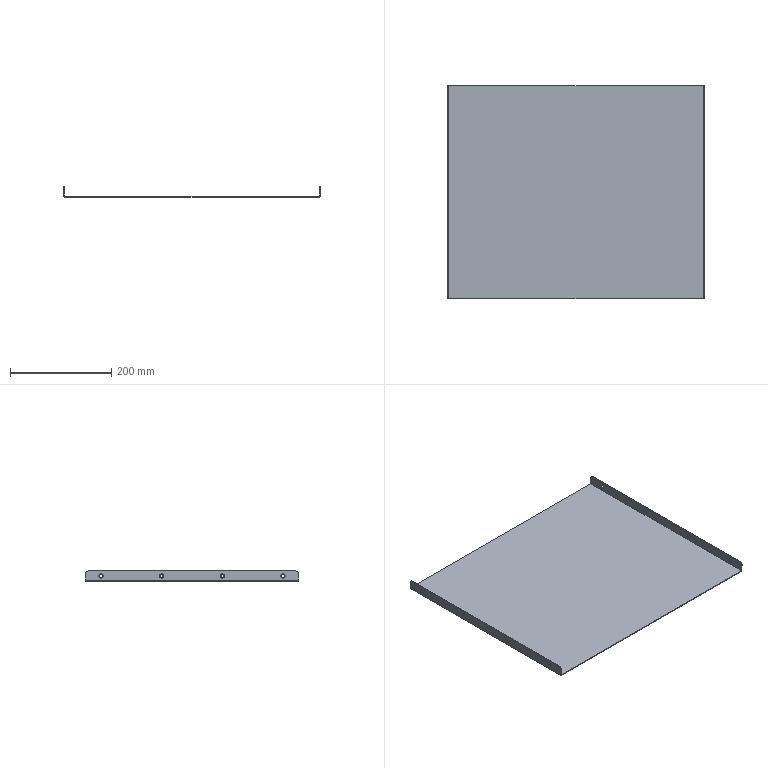Part | SolidWorks | features Chamfer 1, EdgeFlange 1, Fillet 1, FlatPattern 1, ICE 1, SMBaseFlange 1, SheetMetal 1 | 1 solid | 42 faces | box 507 x 421 x 20 mm | volume 342480 mm3 | plane 18 | cone 16 | cylinder 8 | commonest cylinder face diameters 10 x4 0.4 x2 3.4 x2
STEP:
#1=CARTESIAN_POINT('',(-253.5,180.,5.6));
#2=VERTEX_POINT('',#1);
#3=CARTESIAN_POINT('',(-253.5,180.,11.4));
#4=VERTEX_POINT('',#3);
#5=CARTESIAN_POINT('',(-253.5,180.,8.5));
#6=DIRECTION('',(-1.,0.,0.));
#7=DIRECTION('',(0.,0.,1.));
#8=AXIS2_PLACEMENT_3D('',#5,#6,#7);
#9=CIRCLE('',#8,2.9);
#10=EDGE_CURVE('',#2,#4,#9,.T.);
#11=ORIENTED_EDGE('',*,*,#10,.T.);
#12=CARTESIAN_POINT('',(-252.,180.,12.9));
#13=VERTEX_POINT('',#12);
#14=CARTESIAN_POINT('',(-253.5,180.,11.4));
#15=DIRECTION('',(0.7071,0.,0.7071));
#16=VECTOR('',#15,1000.);
#17=LINE('',#14,#16);
#18=EDGE_CURVE('',#4,#13,#17,.T.);
#19=ORIENTED_EDGE('',*,*,#18,.T.);
#20=CARTESIAN_POINT('',(-252.,180.,4.1));
#21=VERTEX_POINT('',#20);
#22=CARTESIAN_POINT('',(-252.,180.,8.5));
#23=DIRECTION('',(-1.,0.,0.));
#24=DIRECTION('',(0.,0.,-1.));
#25=AXIS2_PLACEMENT_3D('',#22,#23,#24);
#26=CIRCLE('',#25,4.4);
#27=EDGE_CURVE('',#21,#13,#26,.T.);
#28=ORIENTED_EDGE('',*,*,#27,.F.);
#29=CARTESIAN_POINT('',(-253.5,180.,5.6));
#30=DIRECTION('',(0.7071,0.,-0.7071));
#31=VECTOR('',#30,1000.);
#32=LINE('',#29,#31);
#33=EDGE_CURVE('',#2,#21,#32,.T.);
#34=ORIENTED_EDGE('',*,*,#33,.F.);
#35=EDGE_LOOP('',(#11,#19,#28,#34));
#36=FACE_OUTER_BOUND('',#35,.T.);
#37=CARTESIAN_POINT('',(-253.5,180.,8.5));
#38=DIRECTION('',(1.,0.,0.));
#39=DIRECTION('',(0.,0.,-1.));
#40=AXIS2_PLACEMENT_3D('',#37,#38,#39);
#41=CONICAL_SURFACE('',#40,2.9,0.7854);
#42=ADVANCED_FACE('',(#36),#41,.F.);
#43=CARTESIAN_POINT('',(-253.5,-180.,5.6));
#44=VERTEX_POINT('',#43);
#45=CARTESIAN_POINT('',(-253.5,-180.,11.4));
#46=VERTEX_POINT('',#45);
#47=CARTESIAN_POINT('',(-253.5,-180.,8.5));
#48=DIRECTION('',(-1.,0.,0.));
#49=DIRECTION('',(0.,0.,1.));
#50=AXIS2_PLACEMENT_3D('',#47,#48,#49);
#51=CIRCLE('',#50,2.9);
#52=EDGE_CURVE('',#44,#46,#51,.T.);
#53=ORIENTED_EDGE('',*,*,#52,.T.);
#54=CARTESIAN_POINT('',(-252.,-180.,12.9));
#55=VERTEX_POINT('',#54);
#56=CARTESIAN_POINT('',(-253.5,-180.,11.4));
#57=DIRECTION('',(0.7071,0.,0.7071));
#58=VECTOR('',#57,1000.);
#59=LINE('',#56,#58);
#60=EDGE_CURVE('',#46,#55,#59,.T.);
#61=ORIENTED_EDGE('',*,*,#60,.T.);
#62=CARTESIAN_POINT('',(-252.,-180.,4.1));
#63=VERTEX_POINT('',#62);
#64=CARTESIAN_POINT('',(-252.,-180.,8.5));
#65=DIRECTION('',(-1.,0.,0.));
#66=DIRECTION('',(0.,0.,-1.));
#67=AXIS2_PLACEMENT_3D('',#64,#65,#66);
#68=CIRCLE('',#67,4.4);
#69=EDGE_CURVE('',#63,#55,#68,.T.);
#70=ORIENTED_EDGE('',*,*,#69,.F.);
#71=CARTESIAN_POINT('',(-253.5,-180.,5.6));
#72=DIRECTION('',(0.7071,0.,-0.7071));
#73=VECTOR('',#72,1000.);
#74=LINE('',#71,#73);
#75=EDGE_CURVE('',#44,#63,#74,.T.);
#76=ORIENTED_EDGE('',*,*,#75,.F.);
#77=EDGE_LOOP('',(#53,#61,#70,#76));
#78=FACE_OUTER_BOUND('',#77,.T.);
#79=CARTESIAN_POINT('',(-253.5,-180.,8.5));
#80=DIRECTION('',(1.,0.,0.));
#81=DIRECTION('',(0.,0.,-1.));
#82=AXIS2_PLACEMENT_3D('',#79,#80,#81);
#83=CONICAL_SURFACE('',#82,2.9,0.7854);
#84=ADVANCED_FACE('',(#78),#83,.F.);
#85=CARTESIAN_POINT('',(253.5,-180.,5.6));
#86=VERTEX_POINT('',#85);
#87=CARTESIAN_POINT('',(253.5,-180.,11.4));
#88=VERTEX_POINT('',#87);
#89=CARTESIAN_POINT('',(253.5,-180.,8.5));
#90=DIRECTION('',(-1.,0.,0.));
#91=DIRECTION('',(0.,0.,1.));
#92=AXIS2_PLACEMENT_3D('',#89,#90,#91);
#93=CIRCLE('',#92,2.9);
#94=EDGE_CURVE('',#86,#88,#93,.T.);
#95=ORIENTED_EDGE('',*,*,#94,.F.);
#96=CARTESIAN_POINT('',(252.,-180.,4.1));
#97=VERTEX_POINT('',#96);
#98=CARTESIAN_POINT('',(252.,-180.,4.1));
#99=DIRECTION('',(-0.7071,0.,-0.7071));
#100=VECTOR('',#99,1000.);
#101=LINE('',#98,#100);
#102=EDGE_CURVE('',#86,#97,#101,.T.);
#103=ORIENTED_EDGE('',*,*,#102,.T.);
#104=CARTESIAN_POINT('',(252.,-180.,12.9));
#105=VERTEX_POINT('',#104);
#106=CARTESIAN_POINT('',(252.,-180.,8.5));
#107=DIRECTION('',(1.,0.,0.));
#108=DIRECTION('',(0.,0.,-1.));
#109=AXIS2_PLACEMENT_3D('',#106,#107,#108);
#110=CIRCLE('',#109,4.4);
#111=EDGE_CURVE('',#105,#97,#110,.T.);
#112=ORIENTED_EDGE('',*,*,#111,.F.);
#113=CARTESIAN_POINT('',(252.,-180.,12.9));
#114=DIRECTION('',(-0.7071,0.,0.7071));
#115=VECTOR('',#114,1000.);
#116=LINE('',#113,#115);
#117=EDGE_CURVE('',#88,#105,#116,.T.);
#118=ORIENTED_EDGE('',*,*,#117,.F.);
#119=EDGE_LOOP('',(#95,#103,#112,#118));
#120=FACE_OUTER_BOUND('',#119,.T.);
#121=CARTESIAN_POINT('',(252.,-180.,8.5));
#122=DIRECTION('',(-1.,0.,0.));
#123=DIRECTION('',(0.,0.,1.));
#124=AXIS2_PLACEMENT_3D('',#121,#122,#123);
#125=CONICAL_SURFACE('',#124,4.4,0.7854);
#126=ADVANCED_FACE('',(#120),#125,.F.);
#127=CARTESIAN_POINT('',(253.5,180.,5.6));
#128=VERTEX_POINT('',#127);
#129=CARTESIAN_POINT('',(253.5,180.,11.4));
#130=VERTEX_POINT('',#129);
#131=CARTESIAN_POINT('',(253.5,180.,8.5));
#132=DIRECTION('',(-1.,0.,0.));
#133=DIRECTION('',(0.,0.,1.));
#134=AXIS2_PLACEMENT_3D('',#131,#132,#133);
#135=CIRCLE('',#134,2.9);
#136=EDGE_CURVE('',#128,#130,#135,.T.);
#137=ORIENTED_EDGE('',*,*,#136,.F.);
#138=CARTESIAN_POINT('',(252.,180.,4.1));
#139=VERTEX_POINT('',#138);
#140=CARTESIAN_POINT('',(252.,180.,4.1));
#141=DIRECTION('',(-0.7071,0.,-0.7071));
#142=VECTOR('',#141,1000.);
#143=LINE('',#140,#142);
#144=EDGE_CURVE('',#128,#139,#143,.T.);
#145=ORIENTED_EDGE('',*,*,#144,.T.);
#146=CARTESIAN_POINT('',(252.,180.,12.9));
#147=VERTEX_POINT('',#146);
#148=CARTESIAN_POINT('',(252.,180.,8.5));
#149=DIRECTION('',(1.,0.,0.));
#150=DIRECTION('',(0.,0.,-1.));
#151=AXIS2_PLACEMENT_3D('',#148,#149,#150);
#152=CIRCLE('',#151,4.4);
#153=EDGE_CURVE('',#147,#139,#152,.T.);
#154=ORIENTED_EDGE('',*,*,#153,.F.);
#155=CARTESIAN_POINT('',(252.,180.,12.9));
#156=DIRECTION('',(-0.7071,0.,0.7071));
#157=VECTOR('',#156,1000.);
#158=LINE('',#155,#157);
#159=EDGE_CURVE('',#130,#147,#158,.T.);
#160=ORIENTED_EDGE('',*,*,#159,.F.);
#161=EDGE_LOOP('',(#137,#145,#154,#160));
#162=FACE_OUTER_BOUND('',#161,.T.);
#163=CARTESIAN_POINT('',(252.,180.,8.5));
#164=DIRECTION('',(-1.,0.,0.));
#165=DIRECTION('',(0.,0.,1.));
#166=AXIS2_PLACEMENT_3D('',#163,#164,#165);
#167=CONICAL_SURFACE('',#166,4.4,0.7854);
#168=ADVANCED_FACE('',(#162),#167,.F.);
#169=CARTESIAN_POINT('',(-253.5,60.,5.6));
#170=VERTEX_POINT('',#169);
#171=CARTESIAN_POINT('',(-253.5,60.,11.4));
#172=VERTEX_POINT('',#171);
#173=CARTESIAN_POINT('',(-253.5,60.,8.5));
#174=DIRECTION('',(-1.,0.,0.));
#175=DIRECTION('',(0.,0.,1.));
#176=AXIS2_PLACEMENT_3D('',#173,#174,#175);
#177=CIRCLE('',#176,2.9);
#178=EDGE_CURVE('',#170,#172,#177,.T.);
#179=ORIENTED_EDGE('',*,*,#178,.T.);
#180=CARTESIAN_POINT('',(-252.,60.,12.9));
#181=VERTEX_POINT('',#180);
#182=CARTESIAN_POINT('',(-253.5,60.,11.4));
#183=DIRECTION('',(0.7071,0.,0.7071));
#184=VECTOR('',#183,1000.);
#185=LINE('',#182,#184);
#186=EDGE_CURVE('',#172,#181,#185,.T.);
#187=ORIENTED_EDGE('',*,*,#186,.T.);
#188=CARTESIAN_POINT('',(-252.,60.,4.1));
#189=VERTEX_POINT('',#188);
#190=CARTESIAN_POINT('',(-252.,60.,8.5));
#191=DIRECTION('',(-1.,0.,0.));
#192=DIRECTION('',(0.,0.,-1.));
#193=AXIS2_PLACEMENT_3D('',#190,#191,#192);
#194=CIRCLE('',#193,4.4);
#195=EDGE_CURVE('',#189,#181,#194,.T.);
#196=ORIENTED_EDGE('',*,*,#195,.F.);
#197=CARTESIAN_POINT('',(-253.5,60.,5.6));
#198=DIRECTION('',(0.7071,0.,-0.7071));
#199=VECTOR('',#198,1000.);
#200=LINE('',#197,#199);
#201=EDGE_CURVE('',#170,#189,#200,.T.);
#202=ORIENTED_EDGE('',*,*,#201,.F.);
#203=EDGE_LOOP('',(#179,#187,#196,#202));
#204=FACE_OUTER_BOUND('',#203,.T.);
#205=CARTESIAN_POINT('',(-253.5,60.,8.5));
#206=DIRECTION('',(1.,0.,0.));
#207=DIRECTION('',(0.,0.,-1.));
#208=AXIS2_PLACEMENT_3D('',#205,#206,#207);
#209=CONICAL_SURFACE('',#208,2.9,0.7854);
#210=ADVANCED_FACE('',(#204),#209,.F.);
#211=CARTESIAN_POINT('',(-253.5,-60.,5.6));
#212=VERTEX_POINT('',#211);
#213=CARTESIAN_POINT('',(-253.5,-60.,11.4));
#214=VERTEX_POINT('',#213);
#215=CARTESIAN_POINT('',(-253.5,-60.,8.5));
#216=DIRECTION('',(-1.,0.,0.));
#217=DIRECTION('',(0.,0.,1.));
#218=AXIS2_PLACEMENT_3D('',#215,#216,#217);
#219=CIRCLE('',#218,2.9);
#220=EDGE_CURVE('',#212,#214,#219,.T.);
#221=ORIENTED_EDGE('',*,*,#220,.T.);
#222=CARTESIAN_POINT('',(-252.,-60.,12.9));
#223=VERTEX_POINT('',#222);
#224=CARTESIAN_POINT('',(-253.5,-60.,11.4));
#225=DIRECTION('',(0.7071,0.,0.7071));
#226=VECTOR('',#225,1000.);
#227=LINE('',#224,#226);
#228=EDGE_CURVE('',#214,#223,#227,.T.);
#229=ORIENTED_EDGE('',*,*,#228,.T.);
#230=CARTESIAN_POINT('',(-252.,-60.,4.1));
#231=VERTEX_POINT('',#230);
#232=CARTESIAN_POINT('',(-252.,-60.,8.5));
#233=DIRECTION('',(-1.,0.,0.));
#234=DIRECTION('',(0.,0.,-1.));
#235=AXIS2_PLACEMENT_3D('',#232,#233,#234);
#236=CIRCLE('',#235,4.4);
#237=EDGE_CURVE('',#231,#223,#236,.T.);
#238=ORIENTED_EDGE('',*,*,#237,.F.);
#239=CARTESIAN_POINT('',(-253.5,-60.,5.6));
#240=DIRECTION('',(0.7071,0.,-0.7071));
#241=VECTOR('',#240,1000.);
#242=LINE('',#239,#241);
#243=EDGE_CURVE('',#212,#231,#242,.T.);
#244=ORIENTED_EDGE('',*,*,#243,.F.);
#245=EDGE_LOOP('',(#221,#229,#238,#244));
#246=FACE_OUTER_BOUND('',#245,.T.);
#247=CARTESIAN_POINT('',(-253.5,-60.,8.5));
#248=DIRECTION('',(1.,0.,0.));
#249=DIRECTION('',(0.,0.,-1.));
#250=AXIS2_PLACEMENT_3D('',#247,#248,#249);
#251=CONICAL_SURFACE('',#250,2.9,0.7854);
#252=ADVANCED_FACE('',(#246),#251,.F.);
#253=CARTESIAN_POINT('',(253.5,60.,5.6));
#254=VERTEX_POINT('',#253);
#255=CARTESIAN_POINT('',(253.5,60.,11.4));
#256=VERTEX_POINT('',#255);
#257=CARTESIAN_POINT('',(253.5,60.,8.5));
#258=DIRECTION('',(-1.,0.,0.));
#259=DIRECTION('',(0.,0.,1.));
#260=AXIS2_PLACEMENT_3D('',#257,#258,#259);
#261=CIRCLE('',#260,2.9);
#262=EDGE_CURVE('',#254,#256,#261,.T.);
#263=ORIENTED_EDGE('',*,*,#262,.F.);
#264=CARTESIAN_POINT('',(252.,60.,4.1));
#265=VERTEX_POINT('',#264);
#266=CARTESIAN_POINT('',(252.,60.,4.1));
#267=DIRECTION('',(-0.7071,0.,-0.7071));
#268=VECTOR('',#267,1000.);
#269=LINE('',#266,#268);
#270=EDGE_CURVE('',#254,#265,#269,.T.);
#271=ORIENTED_EDGE('',*,*,#270,.T.);
#272=CARTESIAN_POINT('',(252.,60.,12.9));
#273=VERTEX_POINT('',#272);
#274=CARTESIAN_POINT('',(252.,60.,8.5));
#275=DIRECTION('',(1.,0.,0.));
#276=DIRECTION('',(0.,0.,-1.));
#277=AXIS2_PLACEMENT_3D('',#274,#275,#276);
#278=CIRCLE('',#277,4.4);
#279=EDGE_CURVE('',#273,#265,#278,.T.);
#280=ORIENTED_EDGE('',*,*,#279,.F.);
#281=CARTESIAN_POINT('',(252.,60.,12.9));
#282=DIRECTION('',(-0.7071,0.,0.7071));
#283=VECTOR('',#282,1000.);
#284=LINE('',#281,#283);
#285=EDGE_CURVE('',#256,#273,#284,.T.);
#286=ORIENTED_EDGE('',*,*,#285,.F.);
#287=EDGE_LOOP('',(#263,#271,#280,#286));
#288=FACE_OUTER_BOUND('',#287,.T.);
#289=CARTESIAN_POINT('',(252.,60.,8.5));
#290=DIRECTION('',(-1.,0.,0.));
#291=DIRECTION('',(0.,0.,1.));
#292=AXIS2_PLACEMENT_3D('',#289,#290,#291);
#293=CONICAL_SURFACE('',#292,4.4,0.7854);
#294=ADVANCED_FACE('',(#288),#293,.F.);
#295=CARTESIAN_POINT('',(252.,-60.,11.4));
#296=VERTEX_POINT('',#295);
#297=CARTESIAN_POINT('',(252.,-60.,5.6));
#298=VERTEX_POINT('',#297);
#299=CARTESIAN_POINT('',(252.,-60.,8.5));
#300=DIRECTION('',(1.,0.,0.));
#301=DIRECTION('',(0.,0.,-1.));
#302=AXIS2_PLACEMENT_3D('',#299,#300,#301);
#303=CIRCLE('',#302,2.9);
#304=EDGE_CURVE('',#296,#298,#303,.T.);
#305=ORIENTED_EDGE('',*,*,#304,.F.);
#306=CARTESIAN_POINT('',(253.5,-60.,12.9));
#307=VERTEX_POINT('',#306);
#308=CARTESIAN_POINT('',(253.5,-60.,12.9));
#309=DIRECTION('',(0.7071,0.,0.7071));
#310=VECTOR('',#309,1000.);
#311=LINE('',#308,#310);
#312=EDGE_CURVE('',#296,#307,#311,.T.);
#313=ORIENTED_EDGE('',*,*,#312,.T.);
#314=CARTESIAN_POINT('',(253.5,-60.,4.1));
#315=VERTEX_POINT('',#314);
#316=CARTESIAN_POINT('',(253.5,-60.,8.5));
#317=DIRECTION('',(-1.,0.,0.));
#318=DIRECTION('',(0.,0.,-1.));
#319=AXIS2_PLACEMENT_3D('',#316,#317,#318);
#320=CIRCLE('',#319,4.4);
#321=EDGE_CURVE('',#315,#307,#320,.T.);
#322=ORIENTED_EDGE('',*,*,#321,.F.);
#323=CARTESIAN_POINT('',(253.5,-60.,4.1));
#324=DIRECTION('',(0.7071,0.,-0.7071));
#325=VECTOR('',#324,1000.);
#326=LINE('',#323,#325);
#327=EDGE_CURVE('',#298,#315,#326,.T.);
#328=ORIENTED_EDGE('',*,*,#327,.F.);
#329=EDGE_LOOP('',(#305,#313,#322,#328));
#330=FACE_OUTER_BOUND('',#329,.T.);
#331=CARTESIAN_POINT('',(253.5,-60.,8.5));
#332=DIRECTION('',(1.,0.,0.));
#333=DIRECTION('',(0.,0.,-1.));
#334=AXIS2_PLACEMENT_3D('',#331,#332,#333);
#335=CONICAL_SURFACE('',#334,4.4,0.7854);
#336=ADVANCED_FACE('',(#330),#335,.F.);
#337=CARTESIAN_POINT('',(-251.8,-210.5,-1.5));
#338=VERTEX_POINT('',#337);
#339=CARTESIAN_POINT('',(-251.8,210.5,-1.5));
#340=VERTEX_POINT('',#339);
#341=CARTESIAN_POINT('',(-251.8,-210.5,-1.5));
#342=DIRECTION('',(0.,1.,0.));
#343=VECTOR('',#342,1000.);
#344=LINE('',#341,#343);
#345=EDGE_CURVE('',#338,#340,#344,.T.);
#346=ORIENTED_EDGE('',*,*,#345,.T.);
#347=CARTESIAN_POINT('',(251.8,210.5,-1.5));
#348=VERTEX_POINT('',#347);
#349=CARTESIAN_POINT('',(-253.5,210.5,-1.5));
#350=DIRECTION('',(-1.,0.,0.));
#351=VECTOR('',#350,1000.);
#352=LINE('',#349,#351);
#353=EDGE_CURVE('',#348,#340,#352,.T.);
#354=ORIENTED_EDGE('',*,*,#353,.F.);
#355=CARTESIAN_POINT('',(251.8,-210.5,-1.5));
#356=VERTEX_POINT('',#355);
#357=CARTESIAN_POINT('',(251.8,210.5,-1.5));
#358=DIRECTION('',(0.,-1.,0.));
#359=VECTOR('',#358,1000.);
#360=LINE('',#357,#359);
#361=EDGE_CURVE('',#348,#356,#360,.T.);
#362=ORIENTED_EDGE('',*,*,#361,.T.);
#363=CARTESIAN_POINT('',(-253.5,-210.5,-1.5));
#364=DIRECTION('',(1.,0.,0.));
#365=VECTOR('',#364,1000.);
#366=LINE('',#363,#365);
#367=EDGE_CURVE('',#338,#356,#366,.T.);
#368=ORIENTED_EDGE('',*,*,#367,.F.);
#369=EDGE_LOOP('',(#346,#354,#362,#368));
#370=FACE_OUTER_BOUND('',#369,.T.);
#371=CARTESIAN_POINT('',(0.,0.,-1.5));
#372=DIRECTION('',(0.,0.,1.));
#373=DIRECTION('',(1.,0.,0.));
#374=AXIS2_PLACEMENT_3D('',#371,#372,#373);
#375=PLANE('',#374);
#376=ADVANCED_FACE('',(#370),#375,.F.);
#377=CARTESIAN_POINT('',(251.8,210.5,0.));
#378=VERTEX_POINT('',#377);
#379=CARTESIAN_POINT('',(-251.8,210.5,0.));
#380=VERTEX_POINT('',#379);
#381=CARTESIAN_POINT('',(-253.5,210.5,0.));
#382=DIRECTION('',(-1.,0.,0.));
#383=VECTOR('',#382,1000.);
#384=LINE('',#381,#383);
#385=EDGE_CURVE('',#378,#380,#384,.T.);
#386=ORIENTED_EDGE('',*,*,#385,.T.);
#387=CARTESIAN_POINT('',(-251.8,-210.5,0.));
#388=VERTEX_POINT('',#387);
#389=CARTESIAN_POINT('',(-251.8,-210.5,0.));
#390=DIRECTION('',(0.,1.,0.));
#391=VECTOR('',#390,1000.);
#392=LINE('',#389,#391);
#393=EDGE_CURVE('',#388,#380,#392,.T.);
#394=ORIENTED_EDGE('',*,*,#393,.F.);
#395=CARTESIAN_POINT('',(251.8,-210.5,0.));
#396=VERTEX_POINT('',#395);
#397=CARTESIAN_POINT('',(-253.5,-210.5,0.));
#398=DIRECTION('',(1.,0.,0.));
#399=VECTOR('',#398,1000.);
#400=LINE('',#397,#399);
#401=EDGE_CURVE('',#388,#396,#400,.T.);
#402=ORIENTED_EDGE('',*,*,#401,.T.);
#403=CARTESIAN_POINT('',(251.8,210.5,0.));
#404=DIRECTION('',(0.,-1.,0.));
#405=VECTOR('',#404,1000.);
#406=LINE('',#403,#405);
#407=EDGE_CURVE('',#378,#396,#406,.T.);
#408=ORIENTED_EDGE('',*,*,#407,.F.);
#409=EDGE_LOOP('',(#386,#394,#402,#408));
#410=FACE_OUTER_BOUND('',#409,.T.);
#411=CARTESIAN_POINT('',(0.,0.,0.));
#412=DIRECTION('',(0.,0.,1.));
#413=DIRECTION('',(1.,0.,0.));
#414=AXIS2_PLACEMENT_3D('',#411,#412,#413);
#415=PLANE('',#414);
#416=ADVANCED_FACE('',(#410),#415,.T.);
#417=ORIENTED_EDGE('',*,*,#401,.F.);
#418=CARTESIAN_POINT('',(-251.8,-210.5,0.));
#419=DIRECTION('',(0.,0.,-1.));
#420=VECTOR('',#419,1000.);
#421=LINE('',#418,#420);
#422=EDGE_CURVE('',#388,#338,#421,.T.);
#423=ORIENTED_EDGE('',*,*,#422,.T.);
#424=ORIENTED_EDGE('',*,*,#367,.T.);
#425=CARTESIAN_POINT('',(251.8,-210.5,0.));
#426=DIRECTION('',(0.,0.,-1.));
#427=VECTOR('',#426,1000.);
#428=LINE('',#425,#427);
#429=EDGE_CURVE('',#396,#356,#428,.T.);
#430=ORIENTED_EDGE('',*,*,#429,.F.);
#431=EDGE_LOOP('',(#417,#423,#424,#430));
#432=FACE_OUTER_BOUND('',#431,.T.);
#433=CARTESIAN_POINT('',(-253.5,-210.5,-1.5));
#434=DIRECTION('',(0.,-1.,0.));
#435=DIRECTION('',(0.,0.,-1.));
#436=AXIS2_PLACEMENT_3D('',#433,#434,#435);
#437=PLANE('',#436);
#438=ADVANCED_FACE('',(#432),#437,.T.);
#439=CARTESIAN_POINT('',(-251.8,210.5,0.));
#440=DIRECTION('',(0.,0.,-1.));
#441=VECTOR('',#440,1000.);
#442=LINE('',#439,#441);
#443=EDGE_CURVE('',#380,#340,#442,.T.);
#444=ORIENTED_EDGE('',*,*,#443,.F.);
#445=ORIENTED_EDGE('',*,*,#385,.F.);
#446=CARTESIAN_POINT('',(251.8,210.5,0.));
#447=DIRECTION('',(0.,0.,-1.));
#448=VECTOR('',#447,1000.);
#449=LINE('',#446,#448);
#450=EDGE_CURVE('',#378,#348,#449,.T.);
#451=ORIENTED_EDGE('',*,*,#450,.T.);
#452=ORIENTED_EDGE('',*,*,#353,.T.);
#453=EDGE_LOOP('',(#444,#445,#451,#452));
#454=FACE_OUTER_BOUND('',#453,.T.);
#455=CARTESIAN_POINT('',(-253.5,210.5,-1.5));
#456=DIRECTION('',(0.,1.,0.));
#457=DIRECTION('',(0.,0.,1.));
#458=AXIS2_PLACEMENT_3D('',#455,#456,#457);
#459=PLANE('',#458);
#460=ADVANCED_FACE('',(#454),#459,.T.);
#461=CARTESIAN_POINT('',(252.,-210.5,0.2));
#462=VERTEX_POINT('',#461);
#463=CARTESIAN_POINT('',(253.5,-210.5,0.2));
#464=VERTEX_POINT('',#463);
#465=CARTESIAN_POINT('',(253.5,-210.5,0.2));
#466=DIRECTION('',(1.,0.,0.));
#467=VECTOR('',#466,1000.);
#468=LINE('',#465,#467);
#469=EDGE_CURVE('',#462,#464,#468,.T.);
#470=ORIENTED_EDGE('',*,*,#469,.F.);
#471=CARTESIAN_POINT('',(251.8,-210.5,0.2));
#472=DIRECTION('',(0.,-1.,0.));
#473=DIRECTION('',(0.,0.,1.));
#474=AXIS2_PLACEMENT_3D('',#471,#472,#473);
#475=CIRCLE('',#474,0.2);
#476=EDGE_CURVE('',#396,#462,#475,.T.);
#477=ORIENTED_EDGE('',*,*,#476,.F.);
#478=ORIENTED_EDGE('',*,*,#429,.T.);
#479=CARTESIAN_POINT('',(251.8,-210.5,0.2));
#480=DIRECTION('',(0.,-1.,0.));
#481=DIRECTION('',(0.,0.,1.));
#482=AXIS2_PLACEMENT_3D('',#479,#480,#481);
#483=CIRCLE('',#482,1.7);
#484=EDGE_CURVE('',#356,#464,#483,.T.);
#485=ORIENTED_EDGE('',*,*,#484,.T.);
#486=EDGE_LOOP('',(#470,#477,#478,#485));
#487=FACE_OUTER_BOUND('',#486,.T.);
#488=CARTESIAN_POINT('',(251.8,-210.5,0.2));
#489=DIRECTION('',(0.,-1.,0.));
#490=DIRECTION('',(0.,0.,-1.));
#491=AXIS2_PLACEMENT_3D('',#488,#489,#490);
#492=PLANE('',#491);
#493=ADVANCED_FACE('',(#487),#492,.T.);
#494=CARTESIAN_POINT('',(252.,210.5,0.2));
#495=VERTEX_POINT('',#494);
#496=CARTESIAN_POINT('',(251.8,210.5,0.2));
#497=DIRECTION('',(0.,1.,0.));
#498=DIRECTION('',(0.,0.,1.));
#499=AXIS2_PLACEMENT_3D('',#496,#497,#498);
#500=CIRCLE('',#499,0.2);
#501=EDGE_CURVE('',#495,#378,#500,.T.);
#502=ORIENTED_EDGE('',*,*,#501,.F.);
#503=CARTESIAN_POINT('',(253.5,210.5,0.2));
#504=VERTEX_POINT('',#503);
#505=CARTESIAN_POINT('',(252.,210.5,0.2));
#506=DIRECTION('',(1.,0.,0.));
#507=VECTOR('',#506,1000.);
#508=LINE('',#505,#507);
#509=EDGE_CURVE('',#495,#504,#508,.T.);
#510=ORIENTED_EDGE('',*,*,#509,.T.);
#511=CARTESIAN_POINT('',(251.8,210.5,0.2));
#512=DIRECTION('',(0.,1.,0.));
#513=DIRECTION('',(0.,0.,1.));
#514=AXIS2_PLACEMENT_3D('',#511,#512,#513);
#515=CIRCLE('',#514,1.7);
#516=EDGE_CURVE('',#504,#348,#515,.T.);
#517=ORIENTED_EDGE('',*,*,#516,.T.);
#518=ORIENTED_EDGE('',*,*,#450,.F.);
#519=EDGE_LOOP('',(#502,#510,#517,#518));
#520=FACE_OUTER_BOUND('',#519,.T.);
#521=CARTESIAN_POINT('',(251.8,210.5,0.2));
#522=DIRECTION('',(0.,-1.,0.));
#523=DIRECTION('',(0.,0.,-1.));
#524=AXIS2_PLACEMENT_3D('',#521,#522,#523);
#525=PLANE('',#524);
#526=ADVANCED_FACE('',(#520),#525,.F.);
#527=ORIENTED_EDGE('',*,*,#361,.F.);
#528=ORIENTED_EDGE('',*,*,#516,.F.);
#529=CARTESIAN_POINT('',(253.5,0.,0.2));
#530=DIRECTION('',(0.,1.,0.));
#531=VECTOR('',#530,1000.);
#532=LINE('',#529,#531);
#533=EDGE_CURVE('',#464,#504,#532,.T.);
#534=ORIENTED_EDGE('',*,*,#533,.F.);
#535=ORIENTED_EDGE('',*,*,#484,.F.);
#536=EDGE_LOOP('',(#527,#528,#534,#535));
#537=FACE_OUTER_BOUND('',#536,.T.);
#538=CARTESIAN_POINT('',(251.8,210.5,0.2));
#539=DIRECTION('',(0.,1.,0.));
#540=DIRECTION('',(1.,0.,0.));
#541=AXIS2_PLACEMENT_3D('',#538,#539,#540);
#542=CYLINDRICAL_SURFACE('',#541,1.7);
#543=ADVANCED_FACE('',(#537),#542,.T.);
#544=ORIENTED_EDGE('',*,*,#407,.T.);
#545=ORIENTED_EDGE('',*,*,#476,.T.);
#546=CARTESIAN_POINT('',(252.,-210.5,0.2));
#547=DIRECTION('',(0.,1.,0.));
#548=VECTOR('',#547,1000.);
#549=LINE('',#546,#548);
#550=EDGE_CURVE('',#462,#495,#549,.T.);
#551=ORIENTED_EDGE('',*,*,#550,.T.);
#552=ORIENTED_EDGE('',*,*,#501,.T.);
#553=EDGE_LOOP('',(#544,#545,#551,#552));
#554=FACE_OUTER_BOUND('',#553,.T.);
#555=CARTESIAN_POINT('',(251.8,210.5,0.2));
#556=DIRECTION('',(0.,1.,0.));
#557=DIRECTION('',(1.,0.,0.));
#558=AXIS2_PLACEMENT_3D('',#555,#556,#557);
#559=CYLINDRICAL_SURFACE('',#558,0.2);
#560=ADVANCED_FACE('',(#554),#559,.F.);
#561=CARTESIAN_POINT('',(252.,210.5,13.5));
#562=VERTEX_POINT('',#561);
#563=CARTESIAN_POINT('',(252.,210.5,0.));
#564=DIRECTION('',(0.,0.,-1.));
#565=VECTOR('',#564,1000.);
#566=LINE('',#563,#565);
#567=EDGE_CURVE('',#562,#495,#566,.T.);
#568=ORIENTED_EDGE('',*,*,#567,.F.);
#569=CARTESIAN_POINT('',(253.5,210.5,13.5));
#570=VERTEX_POINT('',#569);
#571=CARTESIAN_POINT('',(253.5,210.5,13.5));
#572=DIRECTION('',(1.,0.,0.));
#573=VECTOR('',#572,1000.);
#574=LINE('',#571,#573);
#575=EDGE_CURVE('',#562,#570,#574,.T.);
#576=ORIENTED_EDGE('',*,*,#575,.T.);
#577=CARTESIAN_POINT('',(253.5,210.5,0.));
#578=DIRECTION('',(0.,0.,-1.));
#579=VECTOR('',#578,1000.);
#580=LINE('',#577,#579);
#581=EDGE_CURVE('',#570,#504,#580,.T.);
#582=ORIENTED_EDGE('',*,*,#581,.T.);
#583=ORIENTED_EDGE('',*,*,#509,.F.);
#584=EDGE_LOOP('',(#568,#576,#582,#583));
#585=FACE_OUTER_BOUND('',#584,.T.);
#586=CARTESIAN_POINT('',(253.5,210.5,0.));
#587=DIRECTION('',(0.,1.,0.));
#588=DIRECTION('',(0.,0.,1.));
#589=AXIS2_PLACEMENT_3D('',#586,#587,#588);
#590=PLANE('',#589);
#591=ADVANCED_FACE('',(#585),#590,.T.);
#592=CARTESIAN_POINT('',(253.5,-210.5,13.5));
#593=VERTEX_POINT('',#592);
#594=CARTESIAN_POINT('',(253.5,-210.5,18.5));
#595=DIRECTION('',(0.,0.,1.));
#596=VECTOR('',#595,1000.);
#597=LINE('',#594,#596);
#598=EDGE_CURVE('',#464,#593,#597,.T.);
#599=ORIENTED_EDGE('',*,*,#598,.T.);
#600=CARTESIAN_POINT('',(252.,-210.5,13.5));
#601=VERTEX_POINT('',#600);
#602=CARTESIAN_POINT('',(253.5,-210.5,13.5));
#603=DIRECTION('',(-1.,0.,0.));
#604=VECTOR('',#603,1000.);
#605=LINE('',#602,#604);
#606=EDGE_CURVE('',#593,#601,#605,.T.);
#607=ORIENTED_EDGE('',*,*,#606,.T.);
#608=CARTESIAN_POINT('',(252.,-210.5,0.));
#609=DIRECTION('',(0.,0.,1.));
#610=VECTOR('',#609,1000.);
#611=LINE('',#608,#610);
#612=EDGE_CURVE('',#462,#601,#611,.T.);
#613=ORIENTED_EDGE('',*,*,#612,.F.);
#614=ORIENTED_EDGE('',*,*,#469,.T.);
#615=EDGE_LOOP('',(#599,#607,#613,#614));
#616=FACE_OUTER_BOUND('',#615,.T.);
#617=CARTESIAN_POINT('',(253.5,-210.5,18.5));
#618=DIRECTION('',(0.,-1.,0.));
#619=DIRECTION('',(0.,0.,-1.));
#620=AXIS2_PLACEMENT_3D('',#617,#618,#619);
#621=PLANE('',#620);
#622=ADVANCED_FACE('',(#616),#621,.T.);
#623=ORIENTED_EDGE('',*,*,#321,.T.);
#624=CARTESIAN_POINT('',(253.5,-60.,8.5));
#625=DIRECTION('',(-1.,0.,0.));
#626=DIRECTION('',(0.,0.,-1.));
#627=AXIS2_PLACEMENT_3D('',#624,#625,#626);
#628=CIRCLE('',#627,4.4);
#629=EDGE_CURVE('',#307,#315,#628,.T.);
#630=ORIENTED_EDGE('',*,*,#629,.T.);
#631=EDGE_LOOP('',(#623,#630));
#632=FACE_BOUND('',#631,.T.);
#633=CARTESIAN_POINT('',(253.5,-180.,8.5));
#634=DIRECTION('',(-1.,0.,0.));
#635=DIRECTION('',(0.,0.,1.));
#636=AXIS2_PLACEMENT_3D('',#633,#634,#635);
#637=CIRCLE('',#636,2.9);
#638=EDGE_CURVE('',#88,#86,#637,.T.);
#639=ORIENTED_EDGE('',*,*,#638,.T.);
#640=ORIENTED_EDGE('',*,*,#94,.T.);
#641=EDGE_LOOP('',(#639,#640));
#642=FACE_BOUND('',#641,.T.);
#643=CARTESIAN_POINT('',(253.5,60.,8.5));
#644=DIRECTION('',(-1.,0.,0.));
#645=DIRECTION('',(0.,0.,1.));
#646=AXIS2_PLACEMENT_3D('',#643,#644,#645);
#647=CIRCLE('',#646,2.9);
#648=EDGE_CURVE('',#256,#254,#647,.T.);
#649=ORIENTED_EDGE('',*,*,#648,.T.);
#650=ORIENTED_EDGE('',*,*,#262,.T.);
#651=EDGE_LOOP('',(#649,#650));
#652=FACE_BOUND('',#651,.T.);
#653=CARTESIAN_POINT('',(253.5,180.,8.5));
#654=DIRECTION('',(-1.,0.,0.));
#655=DIRECTION('',(0.,0.,1.));
#656=AXIS2_PLACEMENT_3D('',#653,#654,#655);
#657=CIRCLE('',#656,2.9);
#658=EDGE_CURVE('',#130,#128,#657,.T.);
#659=ORIENTED_EDGE('',*,*,#658,.T.);
#660=ORIENTED_EDGE('',*,*,#136,.T.);
#661=EDGE_LOOP('',(#659,#660));
#662=FACE_BOUND('',#661,.T.);
#663=ORIENTED_EDGE('',*,*,#581,.F.);
#664=CARTESIAN_POINT('',(253.5,205.5,18.5));
#665=VERTEX_POINT('',#664);
#666=CARTESIAN_POINT('',(253.5,205.5,13.5));
#667=DIRECTION('',(1.,0.,0.));
#668=DIRECTION('',(0.,0.,-1.));
#669=AXIS2_PLACEMENT_3D('',#666,#667,#668);
#670=CIRCLE('',#669,5.);
#671=EDGE_CURVE('',#570,#665,#670,.T.);
#672=ORIENTED_EDGE('',*,*,#671,.T.);
#673=CARTESIAN_POINT('',(253.5,-205.5,18.5));
#674=VERTEX_POINT('',#673);
#675=CARTESIAN_POINT('',(253.5,210.5,18.5));
#676=DIRECTION('',(0.,1.,0.));
#677=VECTOR('',#676,1000.);
#678=LINE('',#675,#677);
#679=EDGE_CURVE('',#674,#665,#678,.T.);
#680=ORIENTED_EDGE('',*,*,#679,.F.);
#681=CARTESIAN_POINT('',(253.5,-205.5,13.5));
#682=DIRECTION('',(1.,0.,0.));
#683=DIRECTION('',(0.,0.,-1.));
#684=AXIS2_PLACEMENT_3D('',#681,#682,#683);
#685=CIRCLE('',#684,5.);
#686=EDGE_CURVE('',#674,#593,#685,.T.);
#687=ORIENTED_EDGE('',*,*,#686,.T.);
#688=ORIENTED_EDGE('',*,*,#598,.F.);
#689=ORIENTED_EDGE('',*,*,#533,.T.);
#690=EDGE_LOOP('',(#663,#672,#680,#687,#688,#689));
#691=FACE_OUTER_BOUND('',#690,.T.);
#692=CARTESIAN_POINT('',(253.5,0.,0.));
#693=DIRECTION('',(1.,0.,0.));
#694=DIRECTION('',(0.,0.,-1.));
#695=AXIS2_PLACEMENT_3D('',#692,#693,#694);
#696=PLANE('',#695);
#697=ADVANCED_FACE('',(#632,#642,#652,#662,#691),#696,.T.);
#698=ORIENTED_EDGE('',*,*,#279,.T.);
#699=CARTESIAN_POINT('',(252.,60.,8.5));
#700=DIRECTION('',(1.,0.,0.));
#701=DIRECTION('',(0.,0.,-1.));
#702=AXIS2_PLACEMENT_3D('',#699,#700,#701);
#703=CIRCLE('',#702,4.4);
#704=EDGE_CURVE('',#265,#273,#703,.T.);
#705=ORIENTED_EDGE('',*,*,#704,.T.);
#706=EDGE_LOOP('',(#698,#705));
#707=FACE_BOUND('',#706,.T.);
#708=ORIENTED_EDGE('',*,*,#153,.T.);
#709=CARTESIAN_POINT('',(252.,180.,8.5));
#710=DIRECTION('',(1.,0.,0.));
#711=DIRECTION('',(0.,0.,-1.));
#712=AXIS2_PLACEMENT_3D('',#709,#710,#711);
#713=CIRCLE('',#712,4.4);
#714=EDGE_CURVE('',#139,#147,#713,.T.);
#715=ORIENTED_EDGE('',*,*,#714,.T.);
#716=EDGE_LOOP('',(#708,#715));
#717=FACE_BOUND('',#716,.T.);
#718=ORIENTED_EDGE('',*,*,#111,.T.);
#719=CARTESIAN_POINT('',(252.,-180.,8.5));
#720=DIRECTION('',(1.,0.,0.));
#721=DIRECTION('',(0.,0.,-1.));
#722=AXIS2_PLACEMENT_3D('',#719,#720,#721);
#723=CIRCLE('',#722,4.4);
#724=EDGE_CURVE('',#97,#105,#723,.T.);
#725=ORIENTED_EDGE('',*,*,#724,.T.);
#726=EDGE_LOOP('',(#718,#725));
#727=FACE_BOUND('',#726,.T.);
#728=CARTESIAN_POINT('',(252.,-60.,8.5));
#729=DIRECTION('',(1.,0.,0.));
#730=DIRECTION('',(0.,0.,-1.));
#731=AXIS2_PLACEMENT_3D('',#728,#729,#730);
#732=CIRCLE('',#731,2.9);
#733=EDGE_CURVE('',#298,#296,#732,.T.);
#734=ORIENTED_EDGE('',*,*,#733,.T.);
#735=ORIENTED_EDGE('',*,*,#304,.T.);
#736=EDGE_LOOP('',(#734,#735));
#737=FACE_BOUND('',#736,.T.);
#738=CARTESIAN_POINT('',(252.,-205.5,18.5));
#739=VERTEX_POINT('',#738);
#740=CARTESIAN_POINT('',(252.,205.5,18.5));
#741=VERTEX_POINT('',#740);
#742=CARTESIAN_POINT('',(252.,0.,18.5));
#743=DIRECTION('',(0.,1.,0.));
#744=VECTOR('',#743,1000.);
#745=LINE('',#742,#744);
#746=EDGE_CURVE('',#739,#741,#745,.T.);
#747=ORIENTED_EDGE('',*,*,#746,.T.);
#748=CARTESIAN_POINT('',(252.,205.5,13.5));
#749=DIRECTION('',(-1.,0.,0.));
#750=DIRECTION('',(0.,0.,-1.));
#751=AXIS2_PLACEMENT_3D('',#748,#749,#750);
#752=CIRCLE('',#751,5.);
#753=EDGE_CURVE('',#741,#562,#752,.T.);
#754=ORIENTED_EDGE('',*,*,#753,.T.);
#755=ORIENTED_EDGE('',*,*,#567,.T.);
#756=ORIENTED_EDGE('',*,*,#550,.F.);
#757=ORIENTED_EDGE('',*,*,#612,.T.);
#758=CARTESIAN_POINT('',(252.,-205.5,13.5));
#759=DIRECTION('',(-1.,0.,0.));
#760=DIRECTION('',(0.,0.,-1.));
#761=AXIS2_PLACEMENT_3D('',#758,#759,#760);
#762=CIRCLE('',#761,5.);
#763=EDGE_CURVE('',#601,#739,#762,.T.);
#764=ORIENTED_EDGE('',*,*,#763,.T.);
#765=EDGE_LOOP('',(#747,#754,#755,#756,#757,#764));
#766=FACE_OUTER_BOUND('',#765,.T.);
#767=CARTESIAN_POINT('',(252.,0.,0.));
#768=DIRECTION('',(1.,0.,0.));
#769=DIRECTION('',(0.,0.,-1.));
#770=AXIS2_PLACEMENT_3D('',#767,#768,#769);
#771=PLANE('',#770);
#772=ADVANCED_FACE('',(#707,#717,#727,#737,#766),#771,.F.);
#773=ORIENTED_EDGE('',*,*,#679,.T.);
#774=CARTESIAN_POINT('',(253.5,205.5,18.5));
#775=DIRECTION('',(-1.,0.,0.));
#776=VECTOR('',#775,1000.);
#777=LINE('',#774,#776);
#778=EDGE_CURVE('',#665,#741,#777,.T.);
#779=ORIENTED_EDGE('',*,*,#778,.T.);
#780=ORIENTED_EDGE('',*,*,#746,.F.);
#781=CARTESIAN_POINT('',(253.5,-205.5,18.5));
#782=DIRECTION('',(1.,0.,0.));
#783=VECTOR('',#782,1000.);
#784=LINE('',#781,#783);
#785=EDGE_CURVE('',#739,#674,#784,.T.);
#786=ORIENTED_EDGE('',*,*,#785,.T.);
#787=EDGE_LOOP('',(#773,#779,#780,#786));
#788=FACE_OUTER_BOUND('',#787,.T.);
#789=CARTESIAN_POINT('',(253.5,210.5,18.5));
#790=DIRECTION('',(0.,0.,1.));
#791=DIRECTION('',(1.,0.,0.));
#792=AXIS2_PLACEMENT_3D('',#789,#790,#791);
#793=PLANE('',#792);
#794=ADVANCED_FACE('',(#788),#793,.T.);
#795=CARTESIAN_POINT('',(-252.,210.5,0.2));
#796=VERTEX_POINT('',#795);
#797=CARTESIAN_POINT('',(-253.5,210.5,0.2));
#798=VERTEX_POINT('',#797);
#799=CARTESIAN_POINT('',(-253.5,210.5,0.2));
#800=DIRECTION('',(-1.,0.,0.));
#801=VECTOR('',#800,1000.);
#802=LINE('',#799,#801);
#803=EDGE_CURVE('',#796,#798,#802,.T.);
#804=ORIENTED_EDGE('',*,*,#803,.F.);
#805=CARTESIAN_POINT('',(-251.8,210.5,0.2));
#806=DIRECTION('',(0.,1.,0.));
#807=DIRECTION('',(0.,0.,-1.));
#808=AXIS2_PLACEMENT_3D('',#805,#806,#807);
#809=CIRCLE('',#808,0.2);
#810=EDGE_CURVE('',#380,#796,#809,.T.);
#811=ORIENTED_EDGE('',*,*,#810,.F.);
#812=ORIENTED_EDGE('',*,*,#443,.T.);
#813=CARTESIAN_POINT('',(-251.8,210.5,0.2));
#814=DIRECTION('',(0.,1.,0.));
#815=DIRECTION('',(0.,0.,-1.));
#816=AXIS2_PLACEMENT_3D('',#813,#814,#815);
#817=CIRCLE('',#816,1.7);
#818=EDGE_CURVE('',#340,#798,#817,.T.);
#819=ORIENTED_EDGE('',*,*,#818,.T.);
#820=EDGE_LOOP('',(#804,#811,#812,#819));
#821=FACE_OUTER_BOUND('',#820,.T.);
#822=CARTESIAN_POINT('',(-251.8,210.5,0.2));
#823=DIRECTION('',(0.,1.,0.));
#824=DIRECTION('',(0.,0.,1.));
#825=AXIS2_PLACEMENT_3D('',#822,#823,#824);
#826=PLANE('',#825);
#827=ADVANCED_FACE('',(#821),#826,.T.);
#828=CARTESIAN_POINT('',(-252.,-210.5,0.2));
#829=VERTEX_POINT('',#828);
#830=CARTESIAN_POINT('',(-251.8,-210.5,0.2));
#831=DIRECTION('',(0.,-1.,0.));
#832=DIRECTION('',(0.,0.,-1.));
#833=AXIS2_PLACEMENT_3D('',#830,#831,#832);
#834=CIRCLE('',#833,0.2);
#835=EDGE_CURVE('',#829,#388,#834,.T.);
#836=ORIENTED_EDGE('',*,*,#835,.F.);
#837=CARTESIAN_POINT('',(-253.5,-210.5,0.2));
#838=VERTEX_POINT('',#837);
#839=CARTESIAN_POINT('',(-252.,-210.5,0.2));
#840=DIRECTION('',(-1.,0.,0.));
#841=VECTOR('',#840,1000.);
#842=LINE('',#839,#841);
#843=EDGE_CURVE('',#829,#838,#842,.T.);
#844=ORIENTED_EDGE('',*,*,#843,.T.);
#845=CARTESIAN_POINT('',(-251.8,-210.5,0.2));
#846=DIRECTION('',(0.,-1.,0.));
#847=DIRECTION('',(0.,0.,-1.));
#848=AXIS2_PLACEMENT_3D('',#845,#846,#847);
#849=CIRCLE('',#848,1.7);
#850=EDGE_CURVE('',#838,#338,#849,.T.);
#851=ORIENTED_EDGE('',*,*,#850,.T.);
#852=ORIENTED_EDGE('',*,*,#422,.F.);
#853=EDGE_LOOP('',(#836,#844,#851,#852));
#854=FACE_OUTER_BOUND('',#853,.T.);
#855=CARTESIAN_POINT('',(-251.8,-210.5,0.2));
#856=DIRECTION('',(0.,1.,0.));
#857=DIRECTION('',(0.,0.,1.));
#858=AXIS2_PLACEMENT_3D('',#855,#856,#857);
#859=PLANE('',#858);
#860=ADVANCED_FACE('',(#854),#859,.F.);
#861=ORIENTED_EDGE('',*,*,#345,.F.);
#862=ORIENTED_EDGE('',*,*,#850,.F.);
#863=CARTESIAN_POINT('',(-253.5,210.5,0.2));
#864=DIRECTION('',(0.,1.,0.));
#865=VECTOR('',#864,1000.);
#866=LINE('',#863,#865);
#867=EDGE_CURVE('',#838,#798,#866,.T.);
#868=ORIENTED_EDGE('',*,*,#867,.T.);
#869=ORIENTED_EDGE('',*,*,#818,.F.);
#870=EDGE_LOOP('',(#861,#862,#868,#869));
#871=FACE_OUTER_BOUND('',#870,.T.);
#872=CARTESIAN_POINT('',(-251.8,-210.5,0.2));
#873=DIRECTION('',(0.,-1.,0.));
#874=DIRECTION('',(-1.,0.,0.));
#875=AXIS2_PLACEMENT_3D('',#872,#873,#874);
#876=CYLINDRICAL_SURFACE('',#875,1.7);
#877=ADVANCED_FACE('',(#871),#876,.T.);
#878=ORIENTED_EDGE('',*,*,#393,.T.);
#879=ORIENTED_EDGE('',*,*,#810,.T.);
#880=CARTESIAN_POINT('',(-252.,210.5,0.2));
#881=DIRECTION('',(0.,-1.,0.));
#882=VECTOR('',#881,1000.);
#883=LINE('',#880,#882);
#884=EDGE_CURVE('',#796,#829,#883,.T.);
#885=ORIENTED_EDGE('',*,*,#884,.T.);
#886=ORIENTED_EDGE('',*,*,#835,.T.);
#887=EDGE_LOOP('',(#878,#879,#885,#886));
#888=FACE_OUTER_BOUND('',#887,.T.);
#889=CARTESIAN_POINT('',(-251.8,-210.5,0.2));
#890=DIRECTION('',(0.,-1.,0.));
#891=DIRECTION('',(-1.,0.,0.));
#892=AXIS2_PLACEMENT_3D('',#889,#890,#891);
#893=CYLINDRICAL_SURFACE('',#892,0.2);
#894=ADVANCED_FACE('',(#888),#893,.F.);
#895=CARTESIAN_POINT('',(-253.5,210.5,13.5));
#896=VERTEX_POINT('',#895);
#897=CARTESIAN_POINT('',(-253.5,210.5,0.));
#898=DIRECTION('',(0.,0.,1.));
#899=VECTOR('',#898,1000.);
#900=LINE('',#897,#899);
#901=EDGE_CURVE('',#798,#896,#900,.T.);
#902=ORIENTED_EDGE('',*,*,#901,.T.);
#903=CARTESIAN_POINT('',(-252.,210.5,13.5));
#904=VERTEX_POINT('',#903);
#905=CARTESIAN_POINT('',(-253.5,210.5,13.5));
#906=DIRECTION('',(1.,0.,0.));
#907=VECTOR('',#906,1000.);
#908=LINE('',#905,#907);
#909=EDGE_CURVE('',#896,#904,#908,.T.);
#910=ORIENTED_EDGE('',*,*,#909,.T.);
#911=CARTESIAN_POINT('',(-252.,210.5,0.));
#912=DIRECTION('',(0.,0.,1.));
#913=VECTOR('',#912,1000.);
#914=LINE('',#911,#913);
#915=EDGE_CURVE('',#796,#904,#914,.T.);
#916=ORIENTED_EDGE('',*,*,#915,.F.);
#917=ORIENTED_EDGE('',*,*,#803,.T.);
#918=EDGE_LOOP('',(#902,#910,#916,#917));
#919=FACE_OUTER_BOUND('',#918,.T.);
#920=CARTESIAN_POINT('',(-253.5,210.5,0.));
#921=DIRECTION('',(0.,1.,0.));
#922=DIRECTION('',(0.,0.,1.));
#923=AXIS2_PLACEMENT_3D('',#920,#921,#922);
#924=PLANE('',#923);
#925=ADVANCED_FACE('',(#919),#924,.T.);
#926=CARTESIAN_POINT('',(-252.,-210.5,13.5));
#927=VERTEX_POINT('',#926);
#928=CARTESIAN_POINT('',(-252.,-210.5,0.));
#929=DIRECTION('',(0.,0.,-1.));
#930=VECTOR('',#929,1000.);
#931=LINE('',#928,#930);
#932=EDGE_CURVE('',#927,#829,#931,.T.);
#933=ORIENTED_EDGE('',*,*,#932,.F.);
#934=CARTESIAN_POINT('',(-253.5,-210.5,13.5));
#935=VERTEX_POINT('',#934);
#936=CARTESIAN_POINT('',(-253.5,-210.5,13.5));
#937=DIRECTION('',(-1.,0.,0.));
#938=VECTOR('',#937,1000.);
#939=LINE('',#936,#938);
#940=EDGE_CURVE('',#927,#935,#939,.T.);
#941=ORIENTED_EDGE('',*,*,#940,.T.);
#942=CARTESIAN_POINT('',(-253.5,-210.5,18.5));
#943=DIRECTION('',(0.,0.,-1.));
#944=VECTOR('',#943,1000.);
#945=LINE('',#942,#944);
#946=EDGE_CURVE('',#935,#838,#945,.T.);
#947=ORIENTED_EDGE('',*,*,#946,.T.);
#948=ORIENTED_EDGE('',*,*,#843,.F.);
#949=EDGE_LOOP('',(#933,#941,#947,#948));
#950=FACE_OUTER_BOUND('',#949,.T.);
#951=CARTESIAN_POINT('',(-253.5,-210.5,18.5));
#952=DIRECTION('',(0.,-1.,0.));
#953=DIRECTION('',(0.,0.,-1.));
#954=AXIS2_PLACEMENT_3D('',#951,#952,#953);
#955=PLANE('',#954);
#956=ADVANCED_FACE('',(#950),#955,.T.);
#957=ORIENTED_EDGE('',*,*,#220,.F.);
#958=CARTESIAN_POINT('',(-253.5,-60.,8.5));
#959=DIRECTION('',(-1.,0.,0.));
#960=DIRECTION('',(0.,0.,1.));
#961=AXIS2_PLACEMENT_3D('',#958,#959,#960);
#962=CIRCLE('',#961,2.9);
#963=EDGE_CURVE('',#214,#212,#962,.T.);
#964=ORIENTED_EDGE('',*,*,#963,.F.);
#965=EDGE_LOOP('',(#957,#964));
#966=FACE_BOUND('',#965,.T.);
#967=ORIENTED_EDGE('',*,*,#52,.F.);
#968=CARTESIAN_POINT('',(-253.5,-180.,8.5));
#969=DIRECTION('',(-1.,0.,0.));
#970=DIRECTION('',(0.,0.,1.));
#971=AXIS2_PLACEMENT_3D('',#968,#969,#970);
#972=CIRCLE('',#971,2.9);
#973=EDGE_CURVE('',#46,#44,#972,.T.);
#974=ORIENTED_EDGE('',*,*,#973,.F.);
#975=EDGE_LOOP('',(#967,#974));
#976=FACE_BOUND('',#975,.T.);
#977=ORIENTED_EDGE('',*,*,#178,.F.);
#978=CARTESIAN_POINT('',(-253.5,60.,8.5));
#979=DIRECTION('',(-1.,0.,0.));
#980=DIRECTION('',(0.,0.,1.));
#981=AXIS2_PLACEMENT_3D('',#978,#979,#980);
#982=CIRCLE('',#981,2.9);
#983=EDGE_CURVE('',#172,#170,#982,.T.);
#984=ORIENTED_EDGE('',*,*,#983,.F.);
#985=EDGE_LOOP('',(#977,#984));
#986=FACE_BOUND('',#985,.T.);
#987=ORIENTED_EDGE('',*,*,#10,.F.);
#988=CARTESIAN_POINT('',(-253.5,180.,8.5));
#989=DIRECTION('',(-1.,0.,0.));
#990=DIRECTION('',(0.,0.,1.));
#991=AXIS2_PLACEMENT_3D('',#988,#989,#990);
#992=CIRCLE('',#991,2.9);
#993=EDGE_CURVE('',#4,#2,#992,.T.);
#994=ORIENTED_EDGE('',*,*,#993,.F.);
#995=EDGE_LOOP('',(#987,#994));
#996=FACE_BOUND('',#995,.T.);
#997=ORIENTED_EDGE('',*,*,#946,.F.);
#998=CARTESIAN_POINT('',(-253.5,-205.5,18.5));
#999=VERTEX_POINT('',#998);
#1000=CARTESIAN_POINT('',(-253.5,-205.5,13.5));
#1001=DIRECTION('',(-1.,0.,0.));
#1002=DIRECTION('',(0.,0.,-1.));
#1003=AXIS2_PLACEMENT_3D('',#1000,#1001,#1002);
#1004=CIRCLE('',#1003,5.);
#1005=EDGE_CURVE('',#935,#999,#1004,.T.);
#1006=ORIENTED_EDGE('',*,*,#1005,.T.);
#1007=CARTESIAN_POINT('',(-253.5,205.5,18.5));
#1008=VERTEX_POINT('',#1007);
#1009=CARTESIAN_POINT('',(-253.5,210.5,18.5));
#1010=DIRECTION('',(0.,-1.,0.));
#1011=VECTOR('',#1010,1000.);
#1012=LINE('',#1009,#1011);
#1013=EDGE_CURVE('',#1008,#999,#1012,.T.);
#1014=ORIENTED_EDGE('',*,*,#1013,.F.);
#1015=CARTESIAN_POINT('',(-253.5,205.5,13.5));
#1016=DIRECTION('',(-1.,0.,0.));
#1017=DIRECTION('',(0.,0.,-1.));
#1018=AXIS2_PLACEMENT_3D('',#1015,#1016,#1017);
#1019=CIRCLE('',#1018,5.);
#1020=EDGE_CURVE('',#1008,#896,#1019,.T.);
#1021=ORIENTED_EDGE('',*,*,#1020,.T.);
#1022=ORIENTED_EDGE('',*,*,#901,.F.);
#1023=ORIENTED_EDGE('',*,*,#867,.F.);
#1024=EDGE_LOOP('',(#997,#1006,#1014,#1021,#1022,#1023));
#1025=FACE_OUTER_BOUND('',#1024,.T.);
#1026=CARTESIAN_POINT('',(-253.5,0.,0.));
#1027=DIRECTION('',(1.,0.,0.));
#1028=DIRECTION('',(0.,0.,-1.));
#1029=AXIS2_PLACEMENT_3D('',#1026,#1027,#1028);
#1030=PLANE('',#1029);
#1031=ADVANCED_FACE('',(#966,#976,#986,#996,#1025),#1030,.F.);
#1032=ORIENTED_EDGE('',*,*,#237,.T.);
#1033=CARTESIAN_POINT('',(-252.,-60.,8.5));
#1034=DIRECTION('',(-1.,0.,0.));
#1035=DIRECTION('',(0.,0.,-1.));
#1036=AXIS2_PLACEMENT_3D('',#1033,#1034,#1035);
#1037=CIRCLE('',#1036,4.4);
#1038=EDGE_CURVE('',#223,#231,#1037,.T.);
#1039=ORIENTED_EDGE('',*,*,#1038,.T.);
#1040=EDGE_LOOP('',(#1032,#1039));
#1041=FACE_BOUND('',#1040,.T.);
#1042=ORIENTED_EDGE('',*,*,#195,.T.);
#1043=CARTESIAN_POINT('',(-252.,60.,8.5));
#1044=DIRECTION('',(-1.,0.,0.));
#1045=DIRECTION('',(0.,0.,-1.));
#1046=AXIS2_PLACEMENT_3D('',#1043,#1044,#1045);
#1047=CIRCLE('',#1046,4.4);
#1048=EDGE_CURVE('',#181,#189,#1047,.T.);
#1049=ORIENTED_EDGE('',*,*,#1048,.T.);
#1050=EDGE_LOOP('',(#1042,#1049));
#1051=FACE_BOUND('',#1050,.T.);
#1052=ORIENTED_EDGE('',*,*,#69,.T.);
#1053=CARTESIAN_POINT('',(-252.,-180.,8.5));
#1054=DIRECTION('',(-1.,0.,0.));
#1055=DIRECTION('',(0.,0.,-1.));
#1056=AXIS2_PLACEMENT_3D('',#1053,#1054,#1055);
#1057=CIRCLE('',#1056,4.4);
#1058=EDGE_CURVE('',#55,#63,#1057,.T.);
#1059=ORIENTED_EDGE('',*,*,#1058,.T.);
#1060=EDGE_LOOP('',(#1052,#1059));
#1061=FACE_BOUND('',#1060,.T.);
#1062=ORIENTED_EDGE('',*,*,#27,.T.);
#1063=CARTESIAN_POINT('',(-252.,180.,8.5));
#1064=DIRECTION('',(-1.,0.,0.));
#1065=DIRECTION('',(0.,0.,-1.));
#1066=AXIS2_PLACEMENT_3D('',#1063,#1064,#1065);
#1067=CIRCLE('',#1066,4.4);
#1068=EDGE_CURVE('',#13,#21,#1067,.T.);
#1069=ORIENTED_EDGE('',*,*,#1068,.T.);
#1070=EDGE_LOOP('',(#1062,#1069));
#1071=FACE_BOUND('',#1070,.T.);
#1072=CARTESIAN_POINT('',(-252.,205.5,18.5));
#1073=VERTEX_POINT('',#1072);
#1074=CARTESIAN_POINT('',(-252.,-205.5,18.5));
#1075=VERTEX_POINT('',#1074);
#1076=CARTESIAN_POINT('',(-252.,0.,18.5));
#1077=DIRECTION('',(0.,-1.,0.));
#1078=VECTOR('',#1077,1000.);
#1079=LINE('',#1076,#1078);
#1080=EDGE_CURVE('',#1073,#1075,#1079,.T.);
#1081=ORIENTED_EDGE('',*,*,#1080,.T.);
#1082=CARTESIAN_POINT('',(-252.,-205.5,13.5));
#1083=DIRECTION('',(1.,0.,0.));
#1084=DIRECTION('',(0.,0.,-1.));
#1085=AXIS2_PLACEMENT_3D('',#1082,#1083,#1084);
#1086=CIRCLE('',#1085,5.);
#1087=EDGE_CURVE('',#1075,#927,#1086,.T.);
#1088=ORIENTED_EDGE('',*,*,#1087,.T.);
#1089=ORIENTED_EDGE('',*,*,#932,.T.);
#1090=ORIENTED_EDGE('',*,*,#884,.F.);
#1091=ORIENTED_EDGE('',*,*,#915,.T.);
#1092=CARTESIAN_POINT('',(-252.,205.5,13.5));
#1093=DIRECTION('',(1.,0.,0.));
#1094=DIRECTION('',(0.,0.,-1.));
#1095=AXIS2_PLACEMENT_3D('',#1092,#1093,#1094);
#1096=CIRCLE('',#1095,5.);
#1097=EDGE_CURVE('',#904,#1073,#1096,.T.);
#1098=ORIENTED_EDGE('',*,*,#1097,.T.);
#1099=EDGE_LOOP('',(#1081,#1088,#1089,#1090,#1091,#1098));
#1100=FACE_OUTER_BOUND('',#1099,.T.);
#1101=CARTESIAN_POINT('',(-252.,0.,0.));
#1102=DIRECTION('',(1.,0.,0.));
#1103=DIRECTION('',(0.,0.,-1.));
#1104=AXIS2_PLACEMENT_3D('',#1101,#1102,#1103);
#1105=PLANE('',#1104);
#1106=ADVANCED_FACE('',(#1041,#1051,#1061,#1071,#1100),#1105,.T.);
#1107=ORIENTED_EDGE('',*,*,#1013,.T.);
#1108=CARTESIAN_POINT('',(-253.5,-205.5,18.5));
#1109=DIRECTION('',(1.,0.,0.));
#1110=VECTOR('',#1109,1000.);
#1111=LINE('',#1108,#1110);
#1112=EDGE_CURVE('',#999,#1075,#1111,.T.);
#1113=ORIENTED_EDGE('',*,*,#1112,.T.);
#1114=ORIENTED_EDGE('',*,*,#1080,.F.);
#1115=CARTESIAN_POINT('',(-253.5,205.5,18.5));
#1116=DIRECTION('',(-1.,0.,0.));
#1117=VECTOR('',#1116,1000.);
#1118=LINE('',#1115,#1117);
#1119=EDGE_CURVE('',#1073,#1008,#1118,.T.);
#1120=ORIENTED_EDGE('',*,*,#1119,.T.);
#1121=EDGE_LOOP('',(#1107,#1113,#1114,#1120));
#1122=FACE_OUTER_BOUND('',#1121,.T.);
#1123=CARTESIAN_POINT('',(-253.5,210.5,18.5));
#1124=DIRECTION('',(0.,0.,1.));
#1125=DIRECTION('',(1.,0.,0.));
#1126=AXIS2_PLACEMENT_3D('',#1123,#1124,#1125);
#1127=PLANE('',#1126);
#1128=ADVANCED_FACE('',(#1122),#1127,.T.);
#1129=ORIENTED_EDGE('',*,*,#671,.F.);
#1130=ORIENTED_EDGE('',*,*,#575,.F.);
#1131=ORIENTED_EDGE('',*,*,#753,.F.);
#1132=ORIENTED_EDGE('',*,*,#778,.F.);
#1133=EDGE_LOOP('',(#1129,#1130,#1131,#1132));
#1134=FACE_OUTER_BOUND('',#1133,.T.);
#1135=CARTESIAN_POINT('',(253.5,205.5,13.5));
#1136=DIRECTION('',(-1.,0.,0.));
#1137=DIRECTION('',(0.,0.,1.));
#1138=AXIS2_PLACEMENT_3D('',#1135,#1136,#1137);
#1139=CYLINDRICAL_SURFACE('',#1138,5.);
#1140=ADVANCED_FACE('',(#1134),#1139,.T.);
#1141=ORIENTED_EDGE('',*,*,#686,.F.);
#1142=ORIENTED_EDGE('',*,*,#785,.F.);
#1143=ORIENTED_EDGE('',*,*,#763,.F.);
#1144=ORIENTED_EDGE('',*,*,#606,.F.);
#1145=EDGE_LOOP('',(#1141,#1142,#1143,#1144));
#1146=FACE_OUTER_BOUND('',#1145,.T.);
#1147=CARTESIAN_POINT('',(253.5,-205.5,13.5));
#1148=DIRECTION('',(-1.,0.,0.));
#1149=DIRECTION('',(0.,0.,1.));
#1150=AXIS2_PLACEMENT_3D('',#1147,#1148,#1149);
#1151=CYLINDRICAL_SURFACE('',#1150,5.);
#1152=ADVANCED_FACE('',(#1146),#1151,.T.);
#1153=ORIENTED_EDGE('',*,*,#1005,.F.);
#1154=ORIENTED_EDGE('',*,*,#940,.F.);
#1155=ORIENTED_EDGE('',*,*,#1087,.F.);
#1156=ORIENTED_EDGE('',*,*,#1112,.F.);
#1157=EDGE_LOOP('',(#1153,#1154,#1155,#1156));
#1158=FACE_OUTER_BOUND('',#1157,.T.);
#1159=CARTESIAN_POINT('',(-253.5,-205.5,13.5));
#1160=DIRECTION('',(1.,0.,0.));
#1161=DIRECTION('',(0.,0.,-1.));
#1162=AXIS2_PLACEMENT_3D('',#1159,#1160,#1161);
#1163=CYLINDRICAL_SURFACE('',#1162,5.);
#1164=ADVANCED_FACE('',(#1158),#1163,.T.);
#1165=ORIENTED_EDGE('',*,*,#1020,.F.);
#1166=ORIENTED_EDGE('',*,*,#1119,.F.);
#1167=ORIENTED_EDGE('',*,*,#1097,.F.);
#1168=ORIENTED_EDGE('',*,*,#909,.F.);
#1169=EDGE_LOOP('',(#1165,#1166,#1167,#1168));
#1170=FACE_OUTER_BOUND('',#1169,.T.);
#1171=CARTESIAN_POINT('',(-253.5,205.5,13.5));
#1172=DIRECTION('',(1.,0.,0.));
#1173=DIRECTION('',(0.,0.,-1.));
#1174=AXIS2_PLACEMENT_3D('',#1171,#1172,#1173);
#1175=CYLINDRICAL_SURFACE('',#1174,5.);
#1176=ADVANCED_FACE('',(#1170),#1175,.T.);
#1177=ORIENTED_EDGE('',*,*,#312,.F.);
#1178=ORIENTED_EDGE('',*,*,#733,.F.);
#1179=ORIENTED_EDGE('',*,*,#327,.T.);
#1180=ORIENTED_EDGE('',*,*,#629,.F.);
#1181=EDGE_LOOP('',(#1177,#1178,#1179,#1180));
#1182=FACE_OUTER_BOUND('',#1181,.T.);
#1183=CARTESIAN_POINT('',(253.5,-60.,8.5));
#1184=DIRECTION('',(1.,0.,0.));
#1185=DIRECTION('',(0.,0.,-1.));
#1186=AXIS2_PLACEMENT_3D('',#1183,#1184,#1185);
#1187=CONICAL_SURFACE('',#1186,4.4,0.7854);
#1188=ADVANCED_FACE('',(#1182),#1187,.F.);
#1189=ORIENTED_EDGE('',*,*,#270,.F.);
#1190=ORIENTED_EDGE('',*,*,#648,.F.);
#1191=ORIENTED_EDGE('',*,*,#285,.T.);
#1192=ORIENTED_EDGE('',*,*,#704,.F.);
#1193=EDGE_LOOP('',(#1189,#1190,#1191,#1192));
#1194=FACE_OUTER_BOUND('',#1193,.T.);
#1195=CARTESIAN_POINT('',(252.,60.,8.5));
#1196=DIRECTION('',(-1.,0.,0.));
#1197=DIRECTION('',(0.,0.,1.));
#1198=AXIS2_PLACEMENT_3D('',#1195,#1196,#1197);
#1199=CONICAL_SURFACE('',#1198,4.4,0.7854);
#1200=ADVANCED_FACE('',(#1194),#1199,.F.);
#1201=ORIENTED_EDGE('',*,*,#228,.F.);
#1202=ORIENTED_EDGE('',*,*,#963,.T.);
#1203=ORIENTED_EDGE('',*,*,#243,.T.);
#1204=ORIENTED_EDGE('',*,*,#1038,.F.);
#1205=EDGE_LOOP('',(#1201,#1202,#1203,#1204));
#1206=FACE_OUTER_BOUND('',#1205,.T.);
#1207=CARTESIAN_POINT('',(-253.5,-60.,8.5));
#1208=DIRECTION('',(1.,0.,0.));
#1209=DIRECTION('',(0.,0.,-1.));
#1210=AXIS2_PLACEMENT_3D('',#1207,#1208,#1209);
#1211=CONICAL_SURFACE('',#1210,2.9,0.7854);
#1212=ADVANCED_FACE('',(#1206),#1211,.F.);
#1213=ORIENTED_EDGE('',*,*,#186,.F.);
#1214=ORIENTED_EDGE('',*,*,#983,.T.);
#1215=ORIENTED_EDGE('',*,*,#201,.T.);
#1216=ORIENTED_EDGE('',*,*,#1048,.F.);
#1217=EDGE_LOOP('',(#1213,#1214,#1215,#1216));
#1218=FACE_OUTER_BOUND('',#1217,.T.);
#1219=CARTESIAN_POINT('',(-253.5,60.,8.5));
#1220=DIRECTION('',(1.,0.,0.));
#1221=DIRECTION('',(0.,0.,-1.));
#1222=AXIS2_PLACEMENT_3D('',#1219,#1220,#1221);
#1223=CONICAL_SURFACE('',#1222,2.9,0.7854);
#1224=ADVANCED_FACE('',(#1218),#1223,.F.);
#1225=ORIENTED_EDGE('',*,*,#144,.F.);
#1226=ORIENTED_EDGE('',*,*,#658,.F.);
#1227=ORIENTED_EDGE('',*,*,#159,.T.);
#1228=ORIENTED_EDGE('',*,*,#714,.F.);
#1229=EDGE_LOOP('',(#1225,#1226,#1227,#1228));
#1230=FACE_OUTER_BOUND('',#1229,.T.);
#1231=CARTESIAN_POINT('',(252.,180.,8.5));
#1232=DIRECTION('',(-1.,0.,0.));
#1233=DIRECTION('',(0.,0.,1.));
#1234=AXIS2_PLACEMENT_3D('',#1231,#1232,#1233);
#1235=CONICAL_SURFACE('',#1234,4.4,0.7854);
#1236=ADVANCED_FACE('',(#1230),#1235,.F.);
#1237=ORIENTED_EDGE('',*,*,#102,.F.);
#1238=ORIENTED_EDGE('',*,*,#638,.F.);
#1239=ORIENTED_EDGE('',*,*,#117,.T.);
#1240=ORIENTED_EDGE('',*,*,#724,.F.);
#1241=EDGE_LOOP('',(#1237,#1238,#1239,#1240));
#1242=FACE_OUTER_BOUND('',#1241,.T.);
#1243=CARTESIAN_POINT('',(252.,-180.,8.5));
#1244=DIRECTION('',(-1.,0.,0.));
#1245=DIRECTION('',(0.,0.,1.));
#1246=AXIS2_PLACEMENT_3D('',#1243,#1244,#1245);
#1247=CONICAL_SURFACE('',#1246,4.4,0.7854);
#1248=ADVANCED_FACE('',(#1242),#1247,.F.);
#1249=ORIENTED_EDGE('',*,*,#60,.F.);
#1250=ORIENTED_EDGE('',*,*,#973,.T.);
#1251=ORIENTED_EDGE('',*,*,#75,.T.);
#1252=ORIENTED_EDGE('',*,*,#1058,.F.);
#1253=EDGE_LOOP('',(#1249,#1250,#1251,#1252));
#1254=FACE_OUTER_BOUND('',#1253,.T.);
#1255=CARTESIAN_POINT('',(-253.5,-180.,8.5));
#1256=DIRECTION('',(1.,0.,0.));
#1257=DIRECTION('',(0.,0.,-1.));
#1258=AXIS2_PLACEMENT_3D('',#1255,#1256,#1257);
#1259=CONICAL_SURFACE('',#1258,2.9,0.7854);
#1260=ADVANCED_FACE('',(#1254),#1259,.F.);
#1261=ORIENTED_EDGE('',*,*,#18,.F.);
#1262=ORIENTED_EDGE('',*,*,#993,.T.);
#1263=ORIENTED_EDGE('',*,*,#33,.T.);
#1264=ORIENTED_EDGE('',*,*,#1068,.F.);
#1265=EDGE_LOOP('',(#1261,#1262,#1263,#1264));
#1266=FACE_OUTER_BOUND('',#1265,.T.);
#1267=CARTESIAN_POINT('',(-253.5,180.,8.5));
#1268=DIRECTION('',(1.,0.,0.));
#1269=DIRECTION('',(0.,0.,-1.));
#1270=AXIS2_PLACEMENT_3D('',#1267,#1268,#1269);
#1271=CONICAL_SURFACE('',#1270,2.9,0.7854);
#1272=ADVANCED_FACE('',(#1266),#1271,.F.);
#1273=CLOSED_SHELL('',(#42,#84,#126,#168,#210,#252,#294,#336,#376,#416,#438,#460,#493,#526,#543,#560,#591,#622,#697,#772,#794,#827,#860,#877,#894,#925,#956,#1031,#1106,#1128,#1140,#1152,#1164,#1176,#1188,#1200,#1212,#1224,#1236,#1248,#1260,#1272));
#1274=MANIFOLD_SOLID_BREP('',#1273);
#1275=CARTESIAN_POINT('',(0.,0.,0.));
#1276=DIRECTION('',(0.,0.,1.));
#1277=DIRECTION('',(1.,0.,0.));
#1278=AXIS2_PLACEMENT_3D('',#1275,#1276,#1277);
#1279=(LENGTH_UNIT()NAMED_UNIT(*)SI_UNIT(.MILLI.,.METRE.));
#1280=UNCERTAINTY_MEASURE_WITH_UNIT(LENGTH_MEASURE(0.00001),#1279,'','');
#1281=(NAMED_UNIT(*)PLANE_ANGLE_UNIT()SI_UNIT($,.RADIAN.));
#1282=(NAMED_UNIT(*)SI_UNIT($,.STERADIAN.)SOLID_ANGLE_UNIT());
#1283=(GEOMETRIC_REPRESENTATION_CONTEXT(3)GLOBAL_UNCERTAINTY_ASSIGNED_CONTEXT((#1280))GLOBAL_UNIT_ASSIGNED_CONTEXT((#1279,#1281,#1282))REPRESENTATION_CONTEXT('',''));
#1284=ADVANCED_BREP_SHAPE_REPRESENTATION('',(#1274,#1278),#1283);